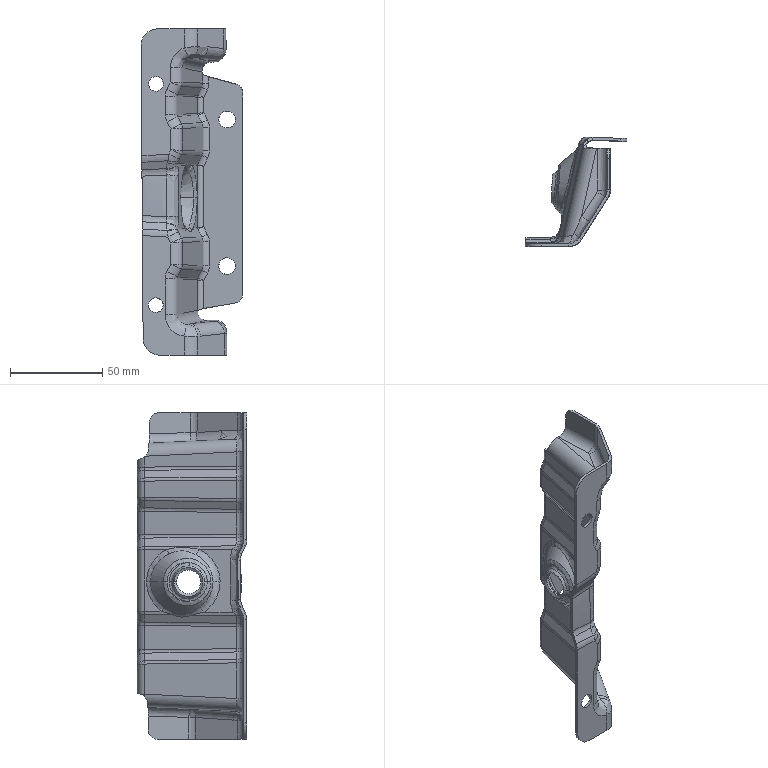Part | STEP file | FNA5401971 | 1 solid | 328 faces | box 55.243 x 59.367 x 177.004 mm | volume 26193 mm3 | spline 183 | cylinder 102 | plane 42 | other 1 | commonest cylinder face diameters 10 x27 13 x16 8 x15 7 x11 14 x8 11 x7